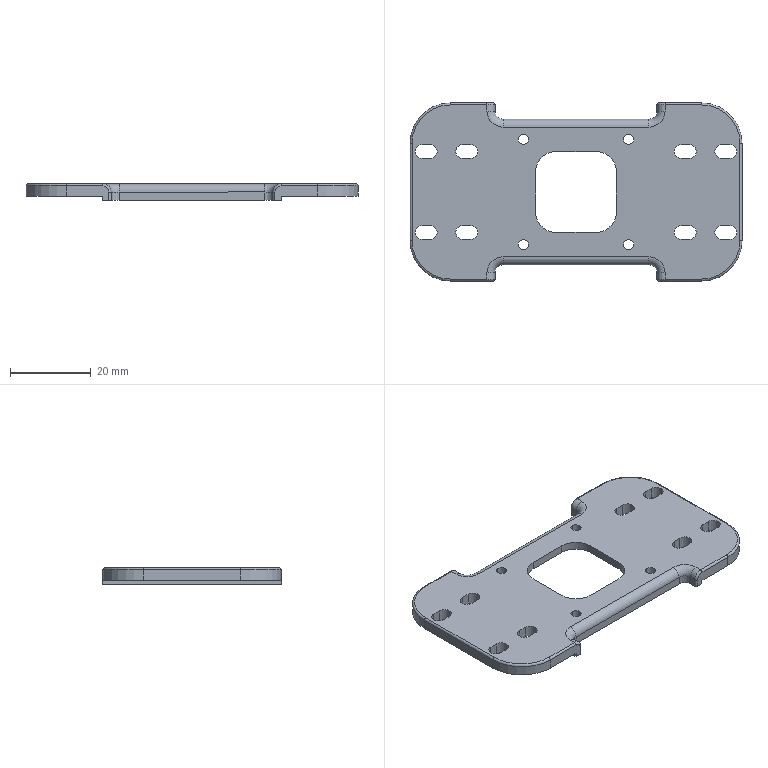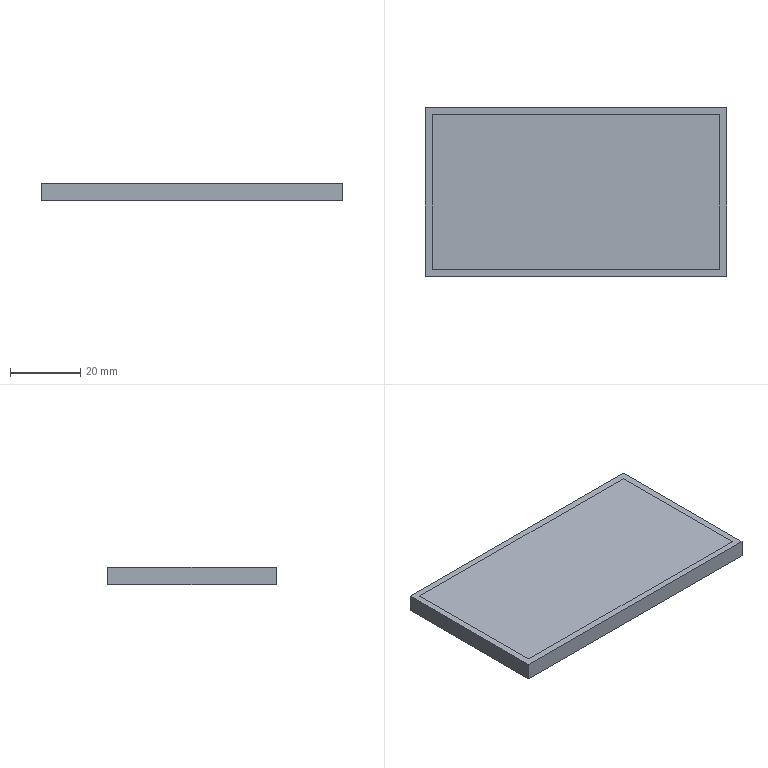CAM job | NX | 3-axis milling, drilling | part box 82 x 44 x 4 mm | stock box 86 x 48 x 5 mm
Tools:
number,name,description,diameter,corner_radius,flute_length,length,flutes
19,D80,Milling Tool-5 Parameters,80.0,0.0,50.0,75.0,2
15,D10,Milling Tool-5 Parameters,10.0,0.0,50.0,75.0,2
14,D10JING,Milling Tool-5 Parameters,10.0,0.0,50.0,75.0,2
1,D6A45,Milling Tool-5 Parameters,6.0,0.0,50.0,75.0,2
2,2.5ZT,Drilling Tool,2.5,0.0,35.0,50.0,2
16,D3,Milling Tool-5 Parameters,3.0,0.0,50.0,75.0,2
18,D3R0.5,Milling Tool-5 Parameters,3.0,0.5,50.0,75.0,2
11,D4,Milling Tool-5 Parameters,4.0,0.0,50.0,75.0,2
Operations:
program,operation,operation_type,tool,method,geometry_group,spindle_rpm,surface_speed,feed_per_tooth,feed_cut,feed_plunge,cut_length_mm,path_length_mm,cut_time_min,machine_time_min
1,FLOOR_WALL,VolumeBased25DMillingOperation,D80,METHOD,A,5000.0,1256.0,0.12,1200.0,100.0,178.0,232.0,0.1483,0.1537
1,ZLEVEL_PROFILE,ZLevelMilling,D10,METHOD,A,9500.0,298.0,0.1842,3500.0,1000.0,1418.141,1478.541,0.4373,0.4433
1,PLANAR_MILL_3,PlanarMilling,D10,METHOD,A,9500.0,298.0,0.1842,3500.0,1000.0,201.337,266.419,0.1322,0.1387
1,ZLEVEL_PROFILE_COPY_COPY,ZLevelMilling,D10JING,METHOD,A,9500.0,298.0,0.0789,1500.0,1000.0,48.63,110.63,0.0339,0.0401
1,SPOT_DRILLING,Operation,D6A45,METHOD,A,9500.0,179.0,0.0132,250.0,0.0,16.0,179.518,0.064,0.0804
1,SPOT_DRILLING_COPY,Operation,2.5ZT,METHOD,A,2500.0,19.0,0.024,120.0,0.0,31.004,209.526,0.2584,0.2762
1,ZLEVEL_PROFILE_COPY_1,ZLevelMilling,D3,METHOD,A,9500.0,89.0,0.0632,1200.0,1000.0,599.024,1200.014,0.5207,0.5808
1,ZLEVEL_PROFILE_COPY_2,ZLevelMilling,D3,METHOD,A,9509.0,89.0,0.071,1350.0,1000.0,669.669,1317.107,0.5476,0.6123
1,ZLEVEL_PROFILE_1_COPY_COPY_COPY,ZLevelMilling,D3R0.5,METHOD,A,9500.0,89.0,0.1316,2500.0,1000.0,2370.477,2520.571,0.9541,0.9691
1,ZLEVEL_PROFILE_1_COPY_COPY_COPY_COPY,ZLevelMilling,D3R0.5,METHOD,A,9500.0,89.0,0.1316,2500.0,1000.0,3314.14,3475.302,1.332,1.348
1,PLANAR_MILL_2_COPY,PlanarMilling,D6A45,METHOD,A,9500.0,179.0,0.0658,1250.0,100.0,221.317,1162.113,0.1771,0.2711
1,ZLEVEL_PROFILE_COPY,ZLevelMilling,D10JING,METHOD,A,9500.0,298.0,0.0632,1200.0,1000.0,1375.246,1440.671,1.147,1.153
2,FLOOR_WALL_COPY,VolumeBased25DMillingOperation,D80,METHOD,B,5000.0,1256.0,0.12,1200.0,100.0,174.0,228.0,0.145,0.1504
2,FLOOR_WALL_1,VolumeBased25DMillingOperation,D4,METHOD,B,9500.0,119.0,0.1316,2500.0,1000.0,2183.038,2423.244,0.892,0.9161
2,FLOOR_WALL_1_COPY,VolumeBased25DMillingOperation,D4,METHOD,B,9500.0,119.0,0.1316,2500.0,700.0,2123.731,2232.176,0.8568,0.8676
2,FLOOR_WALL_1_COPY_COPY,VolumeBased25DMillingOperation,D4,METHOD,B,9500.0,119.0,0.0684,1300.0,700.0,1593.113,1943.8,1.237,1.272
2,ZLEVEL_PROFILE_COPY_1_COPY,ZLevelMilling,D3,METHOD,B,9500.0,89.0,0.0632,1200.0,1000.0,304.88,642.659,0.2649,0.2987
2,PLANAR_MILL_2_COPY_COPY,PlanarMilling,D6A45,METHOD,B,9500.0,179.0,0.0658,1250.0,100.0,402.147,862.896,0.3217,0.3678
2,PLANAR_MILL_2_COPY_COPY_COPY,PlanarMilling,D6A45,METHOD,B,9500.0,179.0,0.0658,1250.0,100.0,72.997,135.997,0.0584,0.0647
2,PLANAR_MILL_2_COPY_COPY_COPY_COPY,PlanarMilling,D6A45,METHOD,B,9500.0,179.0,0.0658,1250.0,100.0,296.396,1077.82,0.2371,0.3153